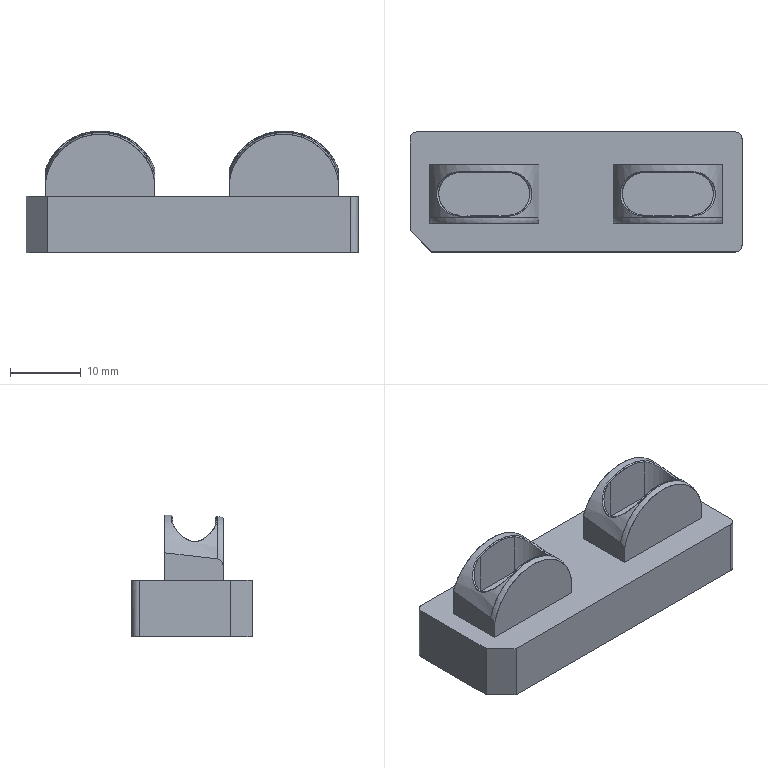CAM job | PowerMill | 3-axis milling, other | part box 47 x 17 x 17.251 mm
Tools:
number,name,type,diameter,tip_radius,length,cutting_length,overhang,flutes,holder,toolpaths_using
1,D10C,end_mill,10.0,0.0,60.0,,30.0,1,D42L35,1
1,D10C_1_1,end_mill,10.0,0.0,60.0,,17.72,1,D42L35,3
15,D3C_1_1,end_mill,3.0,0.0,30.0,,9.44,1,D42L35,1
3,D10_1_1,end_mill,10.0,0.0,60.0,,17.4,1,D42L35,3
22,R1.5_1_1,ball_nosed,3.0,1.5,30.0,,8.12,1,D42L35,1
10,D3_1_1,end_mill,3.0,0.0,30.0,,7.36,1,D42L35,2
13,Text_D4_1_1,taper_spherical,4.0,0.3,60.0,,9.52,1,D42L35,1
Operations:
program,toolpath,strategy,tool,tool_number,tool_diameter,tip_radius,flutes,spindle_rpm,feed_cut,surface_speed_m_min_computed,feed_per_tooth_computed,tolerance,thickness,stepover,stepdown,cut_length,cut_time_min,total_time_min,workplane
23-S-3-F,精公开粗01-扫面平行-D10C,raster_area_clear,D10C_1_1,1,10.0,0.0,1.0,8000.0,10000.0,251.33,1.25,0.03,0.28,6.0,1.0,285.36,0.029,0.035,
23-S-3-F,精公开粗01-外形偏置-D10C,offset_area_clear,D10C_1_1,1,10.0,0.0,1.0,8000.0,10000.0,251.33,1.25,0.03,0.28,6.0,1.0,7144.874,0.715,0.7733,
23-S-3-F,精公开粗01-基准台等高-D10C,constantz,D10C_1_1,1,10.0,0.0,1.0,8000.0,10000.0,251.33,1.25,0.03,0.07,5.0,0.4,3448.961,0.345,0.3546,
23-S-3-F,精公再粗02-外形偏置-D3C,offset_area_clear,D3C_1_1,15,3.0,0.0,1.0,18000.0,5000.0,169.65,0.2778,0.03,0.0,2.0,1.0,10648.731,2.13,2.874,
23-S-3-F,精公基准台01-基准面偏置-D10,offset_area_clear,D10_1_1,3,10.0,0.0,1.0,8500.0,600.0,267.04,0.0706,0.005,0.38,5.0,1.0,144.831,0.241,0.2604,
23-S-3-F,精公基准台01-外形侧光-D10,profile_area_clear,D10_1_1,3,10.0,0.0,1.0,8500.0,600.0,267.04,0.0706,0.005,-0.07,0.08,1.0,314.777,0.525,0.5641,
23-S-3-F,精公基准台01-基准台侧光-D10,profile_area_clear,D10_1_1,3,10.0,0.0,1.0,8500.0,600.0,267.04,0.0706,0.005,0.0,0.08,1.0,313.234,0.522,0.5865,
23-S-3-F,精公精光01-平行-R1.5,raster,R1.5_1_1,22,3.0,1.5,1.0,22000.0,2000.0,207.35,0.0909,0.005,-0.075,0.04,1.0,7890.047,3.945,4.013,
23-S-3-F,精公精光02-等高-D3,constantz,D3_1_1,10,3.0,0.0,1.0,18000.0,2000.0,169.65,0.1111,0.005,-0.075,5.0,0.03,9544.193,4.772,5.124,
23-S-3-F,精公精光02-平坦面平行-D3,raster_area_clear,D3_1_1,10,3.0,0.0,1.0,18000.0,600.0,169.65,0.0333,0.005,0.375,1.5,1.0,94.9,0.158,0.2441,
23-S-3-F,精公刻字01-刻字-Text_D4,pattern,Text_D4_1_1,13,4.0,0.3,1.0,15000.0,1000.0,188.5,0.0667,0.005,0.0,5.0,1.0,40.841,0.041,0.057,
,精公开粗01-外形偏置-D10C_Reference,offset_area_clear,D10C,1,10.0,0.0,1.0,8000.0,10000.0,251.33,1.25,0.03,0.28,6.0,1.0,19022.943,1.902,2.053,